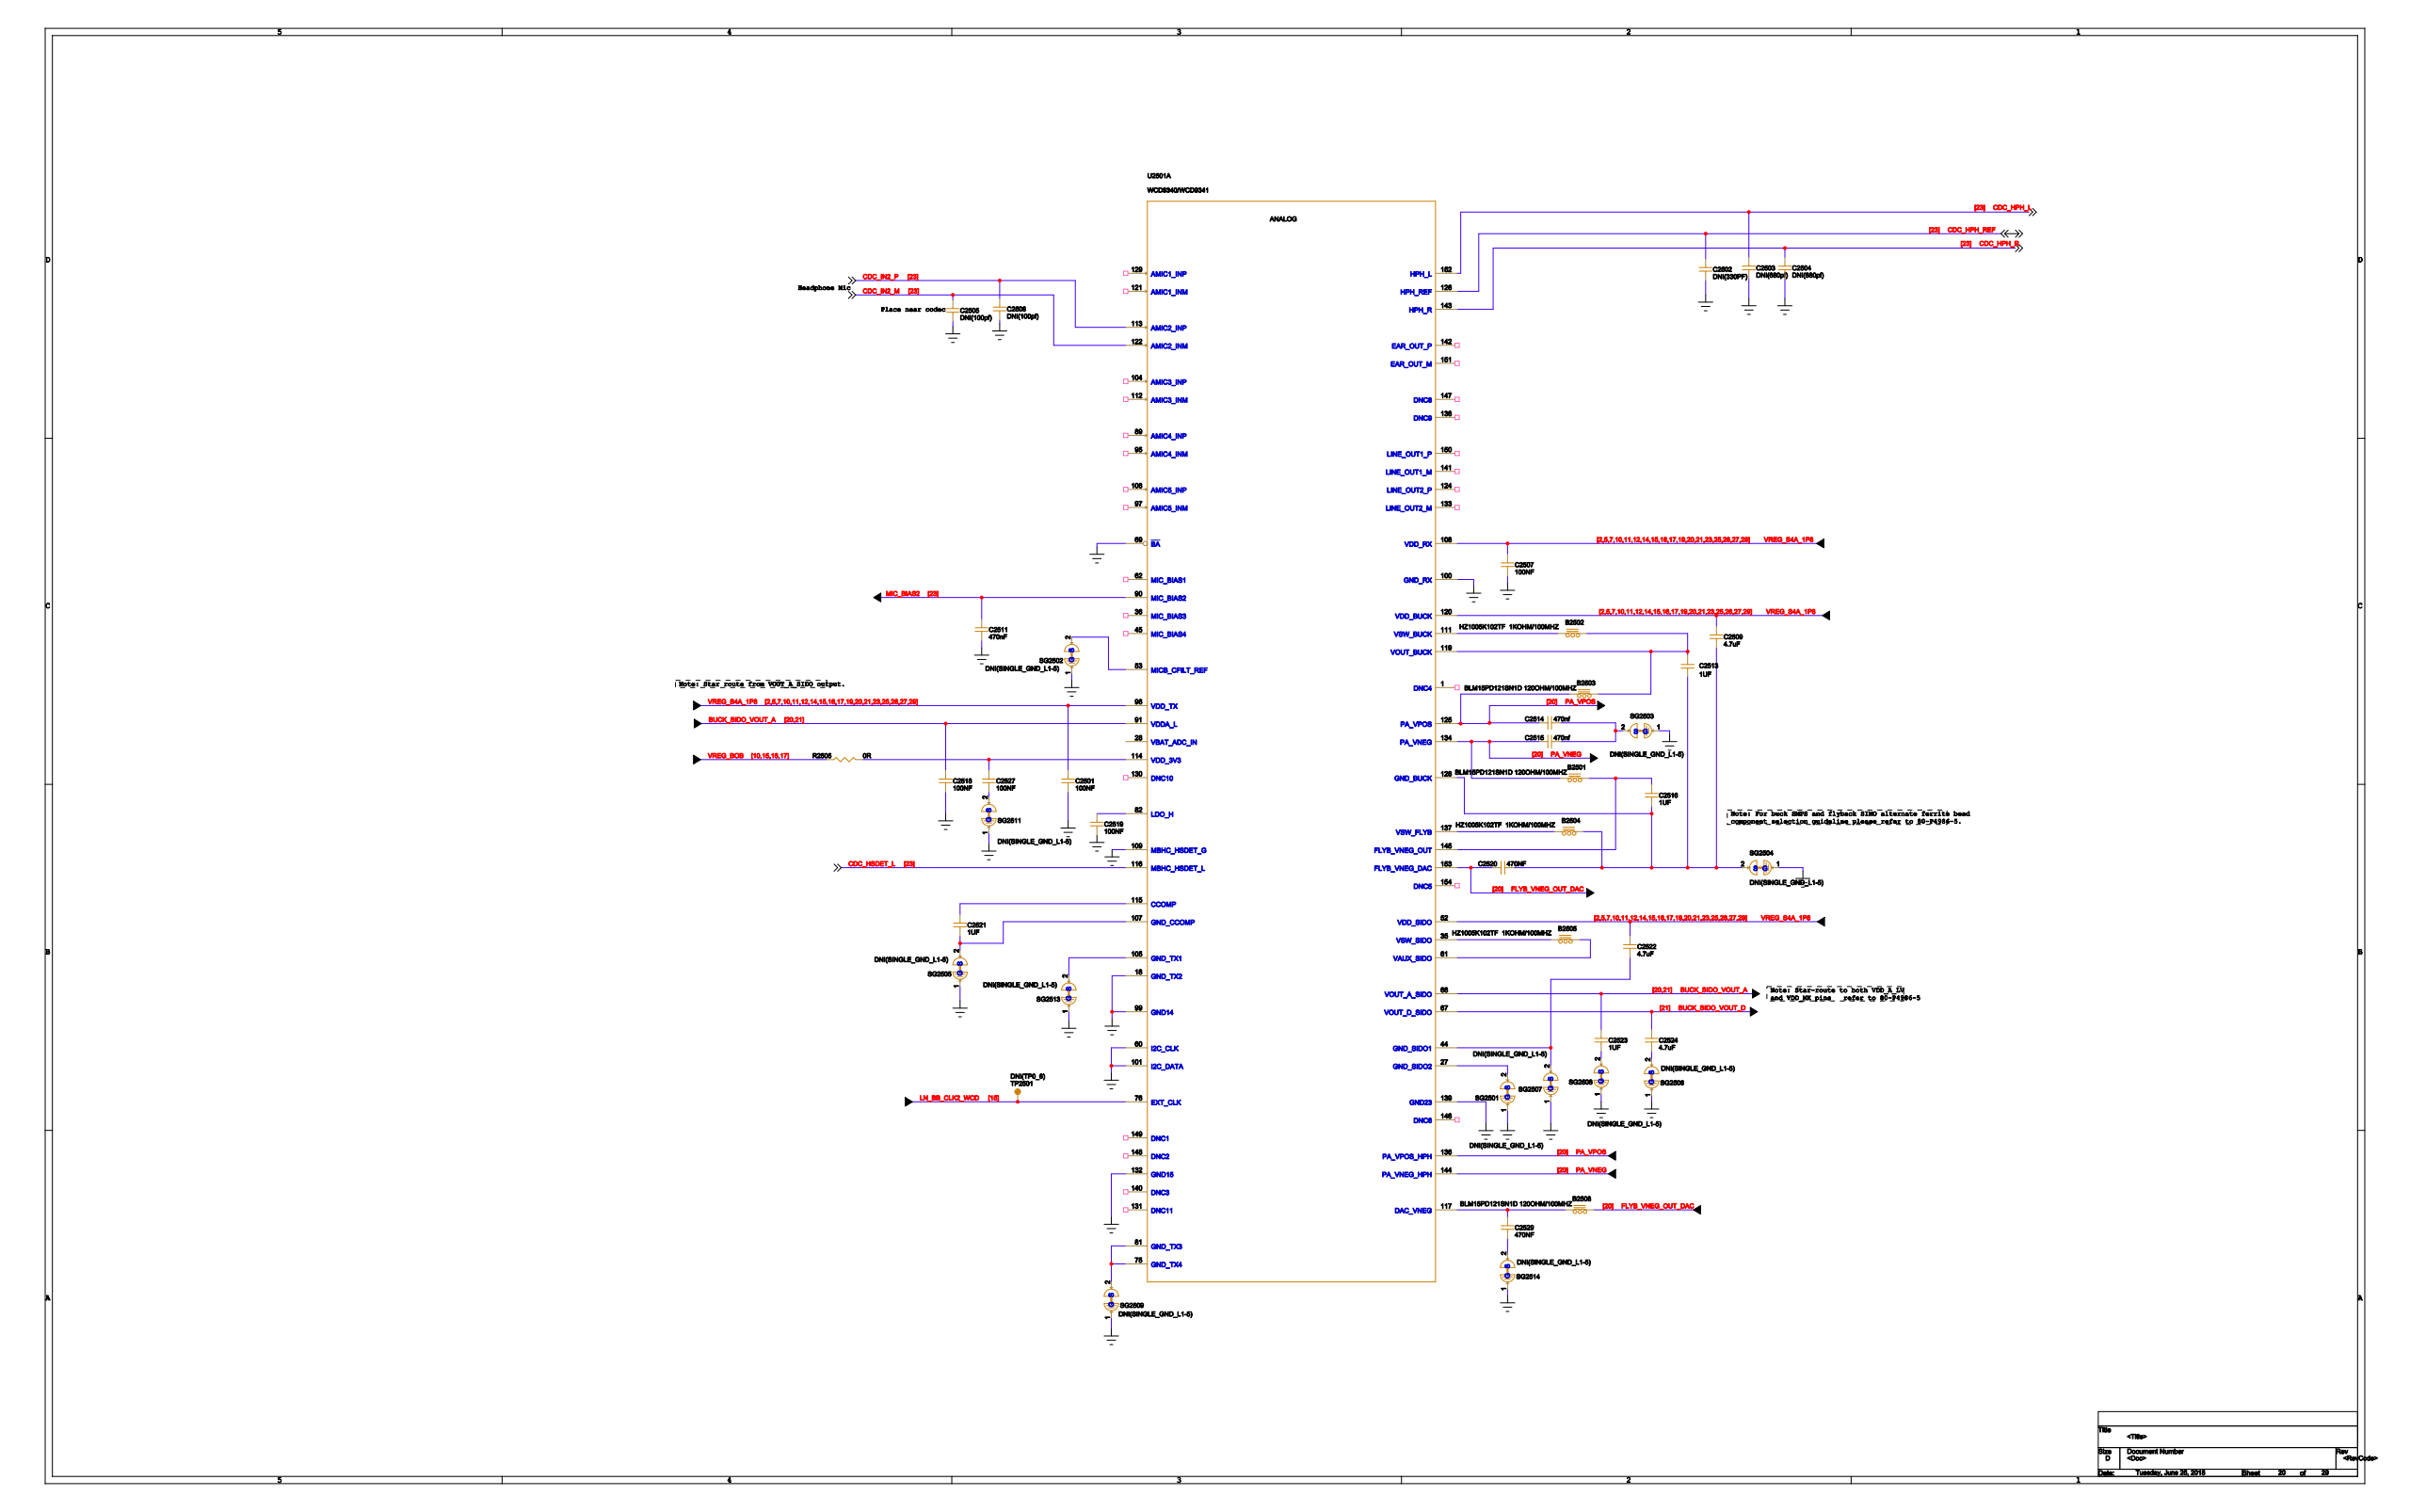Circuit board | Cadence Allegro | 802 parts | 566 nets | one sheet of the schematic
Parts on this sheet (reference | value | footprint):
B2501 | BLM15PD121SN1D 120OHM/100MHZ | BLM15AG121SN1D
B2502 | HZ1005K102TF  1KOHM/100MHZ | FB0402
B2503 | BLM15PD121SN1D 120OHM/100MHZ | BLM15AG121SN1D
B2504 | HZ1005K102TF  1KOHM/100MHZ | FB0402
B2505 | HZ1005K102TF  1KOHM/100MHZ | FB0402
B2508 | BLM15PD121SN1D 120OHM/100MHZ | BLM15AG121SN1D
C2501 | 100NF | C0201
C2502 | DNI(330PF) | C0201
C2503 | DNI(680pf) | C0201
C2504 | DNI(680pf) | C0201
C2505 | DNI(100pf) | C0201
C2506 | DNI(100pf) | C0201
C2507 | 100NF | C0201
C2509 | 4.7uF | 0402-BIG
C2511 | 470nF | C0201
C2513 | 1UF | C0402
C2514 | 470nf | C0402
C2515 | 470nf | C0402
C2516 | 1uF | C0201
C2518 | 100NF | C0201
C2519 | 100NF | C0201
C2520 | 470nF | C0201
C2521 | 1uF | C0201
C2522 | 4.7uF | 0402-BIG
C2523 | 1uF | C0201
C2524 | 4.7uF | 0402-BIG
C2527 | 100NF | C0201
C2529 | 470nF | C0201
R2505 | 0R | R0201
SG2501 | DNI(SINGLE_GND_L1-5) | GND_L1-5
SG2502 | DNI(SINGLE_GND_L1-5) | GND_L1-5
SG2503 | DNI(SINGLE_GND_L1-5) | GND_L1-5
SG2504 | DNI(SINGLE_GND_L1-5) | GND_L1-5
SG2505 | DNI(SINGLE_GND_L1-5) | GND_L1-5
SG2506 | DNI(SINGLE_GND_L1-5) | GND_L1-5
SG2507 | DNI(SINGLE_GND_L1-5) | GND_L1-5
SG2508 | DNI(SINGLE_GND_L1-5) | GND_L1-5
SG2509 | DNI(SINGLE_GND_L1-5) | GND_L1-5
SG2511 | DNI(SINGLE_GND_L1-5) | GND_L1-5
SG2513 | DNI(SINGLE_GND_L1-5) | GND_L1-5
SG2514 | DNI(SINGLE_GND_L1-5) | GND_L1-5
TP2501 | DNI(TP0_6) | TP_C0P6
U2501 | WCD9340/WCD9341 | WLPSP154_4P93X4P30X0P65_0P35
Nets of these parts (net: part-pin ...):
GND: C2501-2 C2502-2 C2503-2 C2504-2 C2505-2 C2506-2 C2507-2 C2511-2 C2518-2 C2519-2 SG2501-1 SG2502-1 SG2503-1 SG2504-1 SG2505-1 SG2506-1 SG2507-1 SG2508-1 SG2509-1 SG2511-1 SG2513-1 SG2514-1 U2501-2 U2501-3 U2501-5 U2501-11 U2501-12 U2501-14 U2501-18 U2501-20 U2501-21 U2501-23 U2501-60 U2501-69 U2501-99 U2501-100 U2501-101 U2501-109 U2501-132 U2501-139
VREG_S4A_1P8: C2501-1 C2507-1 C2509-1 C2522-1 U2501-4 U2501-16 U2501-52 U2501-96 U2501-108 U2501-120
BUCK_SIDO_VOUT_A: C2518-1 C2523-1 U2501-19 U2501-26 U2501-68 U2501-91
N284759: C2519-1 U2501-82
N284919: C2527-1 R2505-2 U2501-114
N323747: C2527-2 SG2511-2
BUCK_SIDO_VOUT_D: C2524-1 U2501-10 U2501-67
CDC_IN2_M: C2505-1 U2501-122
CDC_IN2_P: C2506-1 U2501-113
MIC_BIAS2: C2511-1 U2501-90
FLYB_VNEG_OUT_DAC: B2508-2 C2520-1 U2501-153
N284707: B2504-2 C2509-2 C2513-1 C2516-2 C2520-2 SG2504-2 U2501-128
N284987: B2508-1 C2529-1 U2501-117
N286467: C2529-2 SG2514-2
VREG_BOB: R2505-1
CDC_HPH_L: C2503-1 U2501-152
CDC_HPH_R: C2504-1 U2501-143
CDC_HSDET_L: U2501-116
N284823: B2501-2 C2516-1 U2501-145
N284931: C2521-1 U2501-115
N284927: C2521-2 SG2505-2 U2501-107
N285099: C2523-2 SG2508-2
PA_VNEG: B2501-1 C2515-1 U2501-134 U2501-144
PA_VPOS: B2503-1 C2514-1 U2501-125 U2501-136
N284855: B2502-2 B2503-2 C2513-2 U2501-119
N284851: B2502-1 U2501-111
N319419: B2504-1 U2501-137
N319574: B2505-1 U2501-35
N284615: B2505-2 U2501-61
CDC_HPH_REF: C2502-1 U2501-126
N285577: C2522-2 SG2507-2 U2501-44
N285019: C2524-2 SG2506-2
N284719: C2514-2 C2515-2 SG2503-2
N320240: SG2501-2 U2501-27
N284531: SG2502-2 U2501-53
N284229: SG2509-2 U2501-75 U2501-81
N284947: SG2513-2 U2501-105
LN_BB_CLK2_WCD: TP2501-1 U2501-76
VBAT_ADC_IN: U2501-28